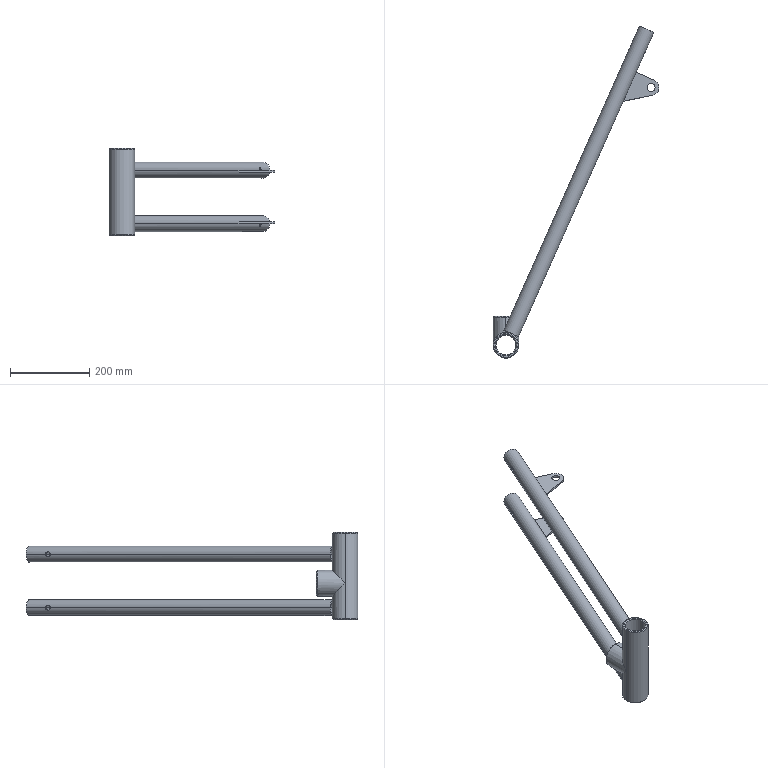Part | SolidWorks | features ICE 5, Chamfer 4, Extrusion 1, MirrorSolid 1, WeldMemberFeat 1, WeldmentFeature 1 | 6 solids | 68 faces | box 418.512 x 837.703 x 220 mm | volume 967255 mm3 | cylinder 37 | plane 19 | cone 12 | commonest cylinder face diameters 13 x8 47 x6 65 x5 20 x4 34 x4 40 x4